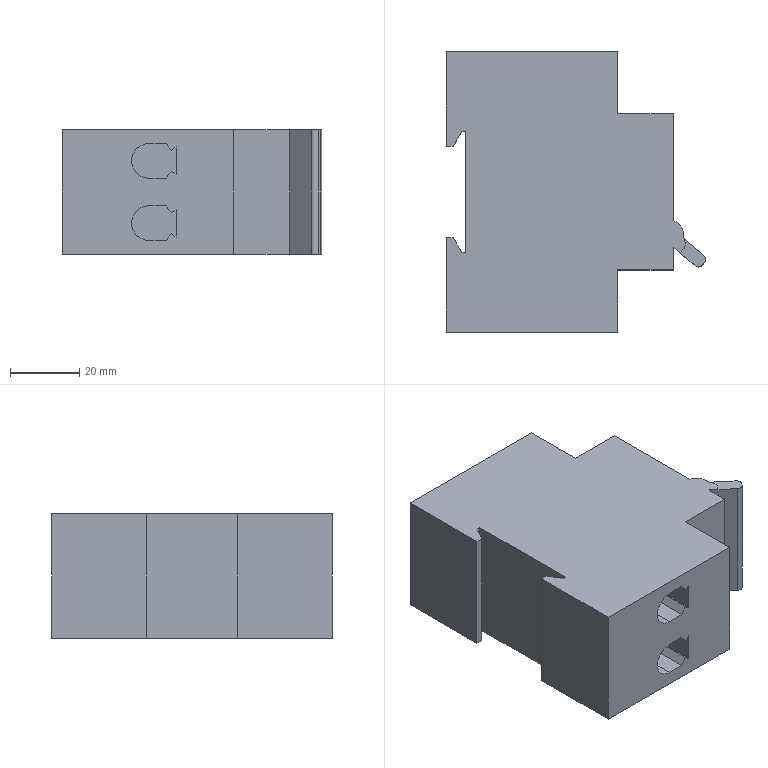Part | SolidWorks | features ICE 7, ConnectionPoint 4, Chamfer 1, CombineBodies 1, Extrusion 1, Fillet 1, LPattern 1, MirrorPattern 1, PLine 1 | 1 solid | 251 faces | box 74.887 x 81 x 36 mm | volume 158863 mm3 | plane 184 | spline 39 | cylinder 28 | commonest cylinder face diameters 7 x8 8.229 x7 5.372 x6 10 x4 3 x3